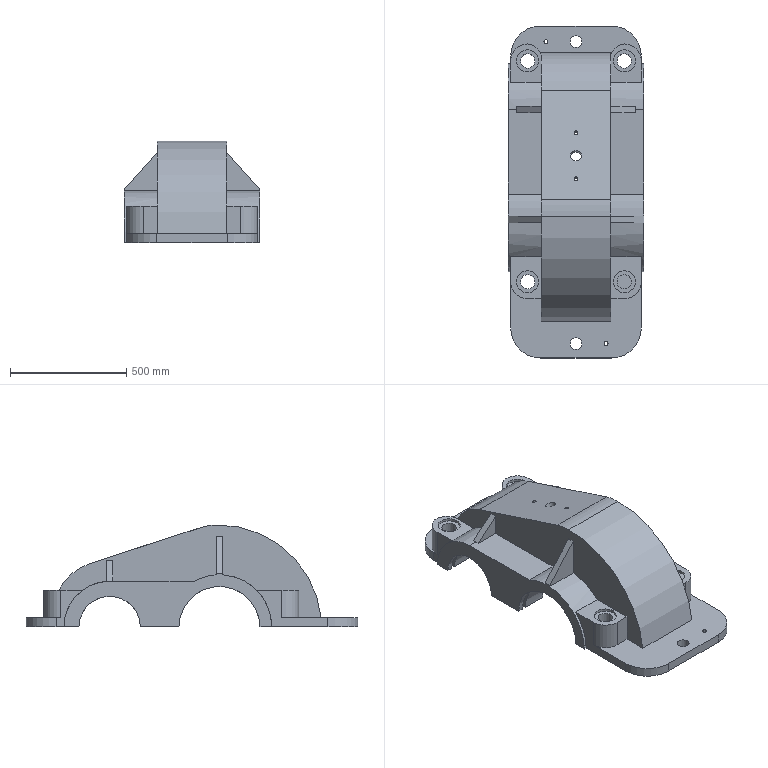Part | NX | features SKETCH 12, BREP 10, Delete Body 6, MOVE_FACE 5, UNITE 5, BLEND 4, DATUM_CSYS 4, EXTRUDE 4, LINKED_BODY 3, REPLACE_FACE 3, SPLIT BODY 3, SUBTRACT 3, SWP104 3, DATUM_PLANE 2, SYMBOLIC_THREAD 2, ABSOLUTE_DATUM_PLANE 1, Container 1, EXTRACT_BODY 1, Geometry Instance 1, LINE 1 | 1 solid | 125 faces | volume 60414139 mm3 | plane 76 | cylinder 49 | commonest cylinder face diameters 146.25 x6 16.875 x4 61.875 x4 95.625 x4 258.75 x4 264.375 x4